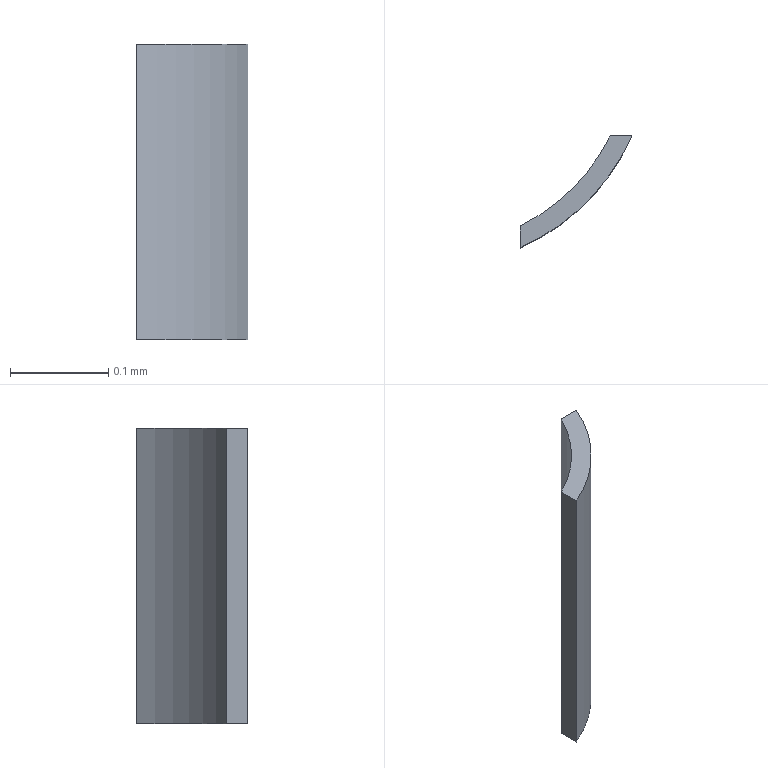Part | STEP file | RJ-USIO-V1_2-220411_172 | 1 solid | 6 faces | box 0.1135 x 0.1135 x 0.3 mm | volume 0.0008879 mm3 | plane 4 | cylinder 2 | commonest cylinder face diameters 0.4 x1 0.44 x1
STEP:
#1=CARTESIAN_POINT('',(0.,0.,0.));
#2=DIRECTION('',(0.,0.,1.));
#3=DIRECTION('',(1.,0.,0.));
#4=AXIS2_PLACEMENT_3D('',#1,#2,#3);
#5=CARTESIAN_POINT('',(38.2,55.808,0.02));
#6=VERTEX_POINT('',#5);
#7=CARTESIAN_POINT('',(38.291,55.9,0.02));
#8=VERTEX_POINT('',#7);
#9=CARTESIAN_POINT('',(38.112,55.988,0.02));
#10=DIRECTION('',(0.,-0.000000044,1.));
#11=DIRECTION('',(0.4406,-0.8977,-0.000000039));
#12=AXIS2_PLACEMENT_3D('',#9,#10,#11);
#13=CIRCLE('',#12,0.2);
#14=CARTESIAN_POINT('',(38.112,55.988,0.02));
#15=DIRECTION('',(0.,-0.000000044,1.));
#16=DIRECTION('',(-0.000000175,1.,0.000000044));
#17=AXIS2_PLACEMENT_3D('',#14,#15,#16);
#18=PLANE('',#17);
#19=CARTESIAN_POINT('',(0.,0.));
#20=DIRECTION('',(-0.8977,-0.4406));
#21=AXIS2_PLACEMENT_2D('',#19,#20);
#22=CIRCLE('',#21,0.2);
#23=(GEOMETRIC_REPRESENTATION_CONTEXT(2)PARAMETRIC_REPRESENTATION_CONTEXT()REPRESENTATION_CONTEXT('',''));
#24=DEFINITIONAL_REPRESENTATION('',(#22),#23);
#25=PCURVE('',#18,#24);
#26=CARTESIAN_POINT('',(38.112,55.988,0.32));
#27=DIRECTION('',(0.,0.000000044,-1.));
#28=DIRECTION('',(0.000000175,-1.,-0.000000044));
#29=AXIS2_PLACEMENT_3D('',#26,#27,#28);
#30=CYLINDRICAL_SURFACE('',#29,0.2);
#31=CARTESIAN_POINT('',(5.827,0.3));
#32=DIRECTION('',(-1.,0.));
#33=VECTOR('',#32,1.);
#34=LINE('',#31,#33);
#35=(GEOMETRIC_REPRESENTATION_CONTEXT(2)PARAMETRIC_REPRESENTATION_CONTEXT()REPRESENTATION_CONTEXT('',''));
#36=DEFINITIONAL_REPRESENTATION('',(#34),#35);
#37=PCURVE('',#30,#36);
#38=SURFACE_CURVE('',#13,(#25,#37),.PCURVE_S1.);
#39=EDGE_CURVE('',#6,#8,#38,.T.);
#40=ORIENTED_EDGE('',*,*,#39,.F.);
#41=CARTESIAN_POINT('',(38.2,55.786,0.02));
#42=VERTEX_POINT('',#41);
#43=CARTESIAN_POINT('',(38.2,55.786,0.02));
#44=DIRECTION('',(-0.000000175,1.,0.000000044));
#45=VECTOR('',#44,1.);
#46=LINE('',#43,#45);
#47=CARTESIAN_POINT('',(-0.2016,-0.08812));
#48=DIRECTION('',(1.,0.));
#49=VECTOR('',#48,1.);
#50=LINE('',#47,#49);
#51=(GEOMETRIC_REPRESENTATION_CONTEXT(2)PARAMETRIC_REPRESENTATION_CONTEXT()REPRESENTATION_CONTEXT('',''));
#52=DEFINITIONAL_REPRESENTATION('',(#50),#51);
#53=PCURVE('',#18,#52);
#54=CARTESIAN_POINT('',(38.2,55.808,0.32));
#55=DIRECTION('',(1.,0.000000175,0.));
#56=DIRECTION('',(0.000000175,-1.,-0.000000044));
#57=AXIS2_PLACEMENT_3D('',#54,#55,#56);
#58=PLANE('',#57);
#59=CARTESIAN_POINT('',(0.02204,0.3));
#60=DIRECTION('',(-1.,0.));
#61=VECTOR('',#60,1.);
#62=LINE('',#59,#61);
#63=(GEOMETRIC_REPRESENTATION_CONTEXT(2)PARAMETRIC_REPRESENTATION_CONTEXT()REPRESENTATION_CONTEXT('',''));
#64=DEFINITIONAL_REPRESENTATION('',(#62),#63);
#65=PCURVE('',#58,#64);
#66=SURFACE_CURVE('',#46,(#53,#65),.PCURVE_S1.);
#67=EDGE_CURVE('',#42,#6,#66,.T.);
#68=ORIENTED_EDGE('',*,*,#67,.F.);
#69=CARTESIAN_POINT('',(38.313,55.9,0.02));
#70=VERTEX_POINT('',#69);
#71=CARTESIAN_POINT('',(38.112,55.988,0.02));
#72=DIRECTION('',(0.,0.000000044,-1.));
#73=DIRECTION('',(0.9163,-0.4005,-0.000000018));
#74=AXIS2_PLACEMENT_3D('',#71,#72,#73);
#75=CIRCLE('',#74,0.22);
#76=CARTESIAN_POINT('',(-0.08812,-0.2016));
#77=CARTESIAN_POINT('',(-0.4373,-0.04895));
#78=CARTESIAN_POINT('',(-0.1305,0.1771));
#79=CARTESIAN_POINT('',(0.1762,0.4032));
#80=CARTESIAN_POINT('',(0.2186,0.02448));
#81=CARTESIAN_POINT('',(0.261,-0.3542));
#82=CARTESIAN_POINT('',(-0.08812,-0.2016));
#83=(BOUNDED_CURVE()B_SPLINE_CURVE(2,(#76,#77,#78,#79,#80,#81,#82),.UNSPECIFIED.,.T.,.F.)B_SPLINE_CURVE_WITH_KNOTS((1,2,2,2,2,1),(-2.094,0.,2.094,4.189,6.283,8.378),.UNSPECIFIED.)CURVE()GEOMETRIC_REPRESENTATION_ITEM()RATIONAL_B_SPLINE_CURVE((1.,0.5,1.,0.5,1.,0.5,1.))REPRESENTATION_ITEM(''));
#84=(GEOMETRIC_REPRESENTATION_CONTEXT(2)PARAMETRIC_REPRESENTATION_CONTEXT()REPRESENTATION_CONTEXT('',''));
#85=DEFINITIONAL_REPRESENTATION('',(#83),#84);
#86=PCURVE('',#18,#85);
#87=CARTESIAN_POINT('',(38.112,55.988,0.32));
#88=DIRECTION('',(0.,0.000000044,-1.));
#89=DIRECTION('',(0.000000175,-1.,-0.000000044));
#90=AXIS2_PLACEMENT_3D('',#87,#88,#89);
#91=CYLINDRICAL_SURFACE('',#90,0.22);
#92=CARTESIAN_POINT('',(5.124,0.3));
#93=DIRECTION('',(1.,0.));
#94=VECTOR('',#93,1.);
#95=LINE('',#92,#94);
#96=(GEOMETRIC_REPRESENTATION_CONTEXT(2)PARAMETRIC_REPRESENTATION_CONTEXT()REPRESENTATION_CONTEXT('',''));
#97=DEFINITIONAL_REPRESENTATION('',(#95),#96);
#98=PCURVE('',#91,#97);
#99=SURFACE_CURVE('',#75,(#86,#98),.PCURVE_S1.);
#100=EDGE_CURVE('',#70,#42,#99,.T.);
#101=ORIENTED_EDGE('',*,*,#100,.F.);
#102=CARTESIAN_POINT('',(38.291,55.9,0.02));
#103=DIRECTION('',(1.,0.000000175,0.));
#104=VECTOR('',#103,1.);
#105=LINE('',#102,#104);
#106=CARTESIAN_POINT('',(-0.08812,-0.1795));
#107=DIRECTION('',(0.,-1.));
#108=VECTOR('',#107,1.);
#109=LINE('',#106,#108);
#110=(GEOMETRIC_REPRESENTATION_CONTEXT(2)PARAMETRIC_REPRESENTATION_CONTEXT()REPRESENTATION_CONTEXT('',''));
#111=DEFINITIONAL_REPRESENTATION('',(#109),#110);
#112=PCURVE('',#18,#111);
#113=CARTESIAN_POINT('',(38.291,55.9,0.32));
#114=DIRECTION('',(0.000000175,-1.,-0.000000044));
#115=DIRECTION('',(-1.,-0.000000175,0.));
#116=AXIS2_PLACEMENT_3D('',#113,#114,#115);
#117=PLANE('',#116);
#118=CARTESIAN_POINT('',(0.,0.3));
#119=DIRECTION('',(-1.,0.));
#120=VECTOR('',#119,1.);
#121=LINE('',#118,#120);
#122=(GEOMETRIC_REPRESENTATION_CONTEXT(2)PARAMETRIC_REPRESENTATION_CONTEXT()REPRESENTATION_CONTEXT('',''));
#123=DEFINITIONAL_REPRESENTATION('',(#121),#122);
#124=PCURVE('',#117,#123);
#125=SURFACE_CURVE('',#105,(#112,#124),.PCURVE_S1.);
#126=EDGE_CURVE('',#8,#70,#125,.T.);
#127=ORIENTED_EDGE('',*,*,#126,.F.);
#128=EDGE_LOOP('',(#40,#68,#101,#127));
#129=FACE_BOUND('',#128,.F.);
#130=ADVANCED_FACE('',(#129),#18,.F.);
#131=ORIENTED_EDGE('',*,*,#39,.T.);
#132=CARTESIAN_POINT('',(38.291,55.9,0.32));
#133=VERTEX_POINT('',#132);
#134=CARTESIAN_POINT('',(38.291,55.9,0.32));
#135=DIRECTION('',(0.,0.000000044,-1.));
#136=VECTOR('',#135,1.);
#137=LINE('',#134,#136);
#138=CARTESIAN_POINT('',(5.169,0.));
#139=DIRECTION('',(0.,1.));
#140=VECTOR('',#139,1.);
#141=LINE('',#138,#140);
#142=(GEOMETRIC_REPRESENTATION_CONTEXT(2)PARAMETRIC_REPRESENTATION_CONTEXT()REPRESENTATION_CONTEXT('',''));
#143=DEFINITIONAL_REPRESENTATION('',(#141),#142);
#144=PCURVE('',#30,#143);
#145=CARTESIAN_POINT('',(0.,0.));
#146=DIRECTION('',(0.,1.));
#147=VECTOR('',#146,1.);
#148=LINE('',#145,#147);
#149=(GEOMETRIC_REPRESENTATION_CONTEXT(2)PARAMETRIC_REPRESENTATION_CONTEXT()REPRESENTATION_CONTEXT('',''));
#150=DEFINITIONAL_REPRESENTATION('',(#148),#149);
#151=PCURVE('',#117,#150);
#152=SURFACE_CURVE('',#137,(#144,#151),.PCURVE_S1.);
#153=EDGE_CURVE('',#133,#8,#152,.T.);
#154=ORIENTED_EDGE('',*,*,#153,.F.);
#155=CARTESIAN_POINT('',(38.2,55.808,0.32));
#156=VERTEX_POINT('',#155);
#157=CARTESIAN_POINT('',(38.112,55.988,0.32));
#158=DIRECTION('',(0.,0.000000044,-1.));
#159=DIRECTION('',(0.8977,-0.4406,-0.000000019));
#160=AXIS2_PLACEMENT_3D('',#157,#158,#159);
#161=CIRCLE('',#160,0.2);
#162=CARTESIAN_POINT('',(5.169,0.));
#163=DIRECTION('',(1.,0.));
#164=VECTOR('',#163,1.);
#165=LINE('',#162,#164);
#166=(GEOMETRIC_REPRESENTATION_CONTEXT(2)PARAMETRIC_REPRESENTATION_CONTEXT()REPRESENTATION_CONTEXT('',''));
#167=DEFINITIONAL_REPRESENTATION('',(#165),#166);
#168=PCURVE('',#30,#167);
#169=CARTESIAN_POINT('',(38.112,55.988,0.32));
#170=DIRECTION('',(0.,-0.000000044,1.));
#171=DIRECTION('',(-0.000000175,1.,0.000000044));
#172=AXIS2_PLACEMENT_3D('',#169,#170,#171);
#173=PLANE('',#172);
#174=CARTESIAN_POINT('',(-0.08812,-0.1795));
#175=CARTESIAN_POINT('',(-0.3991,-0.02691));
#176=CARTESIAN_POINT('',(-0.1114,0.1661));
#177=CARTESIAN_POINT('',(0.1762,0.3591));
#178=CARTESIAN_POINT('',(0.1995,0.01346));
#179=CARTESIAN_POINT('',(0.2229,-0.3322));
#180=CARTESIAN_POINT('',(-0.08812,-0.1795));
#181=(BOUNDED_CURVE()B_SPLINE_CURVE(2,(#174,#175,#176,#177,#178,#179,#180),.UNSPECIFIED.,.T.,.F.)B_SPLINE_CURVE_WITH_KNOTS((1,2,2,2,2,1),(-2.094,0.,2.094,4.189,6.283,8.378),.UNSPECIFIED.)CURVE()GEOMETRIC_REPRESENTATION_ITEM()RATIONAL_B_SPLINE_CURVE((1.,0.5,1.,0.5,1.,0.5,1.))REPRESENTATION_ITEM(''));
#182=(GEOMETRIC_REPRESENTATION_CONTEXT(2)PARAMETRIC_REPRESENTATION_CONTEXT()REPRESENTATION_CONTEXT('',''));
#183=DEFINITIONAL_REPRESENTATION('',(#181),#182);
#184=PCURVE('',#173,#183);
#185=SURFACE_CURVE('',#161,(#168,#184),.PCURVE_S1.);
#186=EDGE_CURVE('',#133,#156,#185,.T.);
#187=ORIENTED_EDGE('',*,*,#186,.T.);
#188=CARTESIAN_POINT('',(38.2,55.808,0.02));
#189=DIRECTION('',(0.,-0.000000044,1.));
#190=VECTOR('',#189,1.);
#191=LINE('',#188,#190);
#192=CARTESIAN_POINT('',(5.827,0.3));
#193=DIRECTION('',(0.,-1.));
#194=VECTOR('',#193,1.);
#195=LINE('',#192,#194);
#196=(GEOMETRIC_REPRESENTATION_CONTEXT(2)PARAMETRIC_REPRESENTATION_CONTEXT()REPRESENTATION_CONTEXT('',''));
#197=DEFINITIONAL_REPRESENTATION('',(#195),#196);
#198=PCURVE('',#30,#197);
#199=CARTESIAN_POINT('',(0.,0.3));
#200=DIRECTION('',(0.,-1.));
#201=VECTOR('',#200,1.);
#202=LINE('',#199,#201);
#203=(GEOMETRIC_REPRESENTATION_CONTEXT(2)PARAMETRIC_REPRESENTATION_CONTEXT()REPRESENTATION_CONTEXT('',''));
#204=DEFINITIONAL_REPRESENTATION('',(#202),#203);
#205=PCURVE('',#58,#204);
#206=SURFACE_CURVE('',#191,(#198,#205),.PCURVE_S1.);
#207=EDGE_CURVE('',#6,#156,#206,.T.);
#208=ORIENTED_EDGE('',*,*,#207,.F.);
#209=EDGE_LOOP('',(#131,#154,#187,#208));
#210=FACE_BOUND('',#209,.F.);
#211=ADVANCED_FACE('',(#210),#30,.F.);
#212=ORIENTED_EDGE('',*,*,#126,.T.);
#213=CARTESIAN_POINT('',(38.313,55.9,0.32));
#214=VERTEX_POINT('',#213);
#215=CARTESIAN_POINT('',(38.313,55.9,0.02));
#216=DIRECTION('',(0.,-0.000000044,1.));
#217=VECTOR('',#216,1.);
#218=LINE('',#215,#217);
#219=CARTESIAN_POINT('',(-0.02204,0.3));
#220=DIRECTION('',(0.,-1.));
#221=VECTOR('',#220,1.);
#222=LINE('',#219,#221);
#223=(GEOMETRIC_REPRESENTATION_CONTEXT(2)PARAMETRIC_REPRESENTATION_CONTEXT()REPRESENTATION_CONTEXT('',''));
#224=DEFINITIONAL_REPRESENTATION('',(#222),#223);
#225=PCURVE('',#117,#224);
#226=CARTESIAN_POINT('',(5.124,0.3));
#227=DIRECTION('',(0.,-1.));
#228=VECTOR('',#227,1.);
#229=LINE('',#226,#228);
#230=(GEOMETRIC_REPRESENTATION_CONTEXT(2)PARAMETRIC_REPRESENTATION_CONTEXT()REPRESENTATION_CONTEXT('',''));
#231=DEFINITIONAL_REPRESENTATION('',(#229),#230);
#232=PCURVE('',#91,#231);
#233=SURFACE_CURVE('',#218,(#225,#232),.PCURVE_S1.);
#234=EDGE_CURVE('',#70,#214,#233,.T.);
#235=ORIENTED_EDGE('',*,*,#234,.T.);
#236=CARTESIAN_POINT('',(38.291,55.9,0.32));
#237=DIRECTION('',(1.,0.000000175,0.));
#238=VECTOR('',#237,1.);
#239=LINE('',#236,#238);
#240=CARTESIAN_POINT('',(0.,0.));
#241=DIRECTION('',(-1.,0.));
#242=VECTOR('',#241,1.);
#243=LINE('',#240,#242);
#244=(GEOMETRIC_REPRESENTATION_CONTEXT(2)PARAMETRIC_REPRESENTATION_CONTEXT()REPRESENTATION_CONTEXT('',''));
#245=DEFINITIONAL_REPRESENTATION('',(#243),#244);
#246=PCURVE('',#117,#245);
#247=CARTESIAN_POINT('',(-0.08812,-0.1795));
#248=DIRECTION('',(0.,-1.));
#249=VECTOR('',#248,1.);
#250=LINE('',#247,#249);
#251=(GEOMETRIC_REPRESENTATION_CONTEXT(2)PARAMETRIC_REPRESENTATION_CONTEXT()REPRESENTATION_CONTEXT('',''));
#252=DEFINITIONAL_REPRESENTATION('',(#250),#251);
#253=PCURVE('',#173,#252);
#254=SURFACE_CURVE('',#239,(#246,#253),.PCURVE_S1.);
#255=EDGE_CURVE('',#133,#214,#254,.T.);
#256=ORIENTED_EDGE('',*,*,#255,.F.);
#257=ORIENTED_EDGE('',*,*,#153,.T.);
#258=EDGE_LOOP('',(#212,#235,#256,#257));
#259=FACE_BOUND('',#258,.F.);
#260=ADVANCED_FACE('',(#259),#117,.F.);
#261=ORIENTED_EDGE('',*,*,#234,.T.);
#262=CARTESIAN_POINT('',(38.2,55.786,0.32));
#263=VERTEX_POINT('',#262);
#264=CARTESIAN_POINT('',(38.112,55.988,0.32));
#265=DIRECTION('',(0.,-0.000000044,1.));
#266=DIRECTION('',(0.4005,-0.9163,-0.00000004));
#267=AXIS2_PLACEMENT_3D('',#264,#265,#266);
#268=CIRCLE('',#267,0.22);
#269=CARTESIAN_POINT('',(5.871,0.));
#270=DIRECTION('',(-1.,0.));
#271=VECTOR('',#270,1.);
#272=LINE('',#269,#271);
#273=(GEOMETRIC_REPRESENTATION_CONTEXT(2)PARAMETRIC_REPRESENTATION_CONTEXT()REPRESENTATION_CONTEXT('',''));
#274=DEFINITIONAL_REPRESENTATION('',(#272),#273);
#275=PCURVE('',#91,#274);
#276=CARTESIAN_POINT('',(0.,0.));
#277=DIRECTION('',(-0.9163,-0.4005));
#278=AXIS2_PLACEMENT_2D('',#276,#277);
#279=CIRCLE('',#278,0.22);
#280=(GEOMETRIC_REPRESENTATION_CONTEXT(2)PARAMETRIC_REPRESENTATION_CONTEXT()REPRESENTATION_CONTEXT('',''));
#281=DEFINITIONAL_REPRESENTATION('',(#279),#280);
#282=PCURVE('',#173,#281);
#283=SURFACE_CURVE('',#268,(#275,#282),.PCURVE_S1.);
#284=EDGE_CURVE('',#263,#214,#283,.T.);
#285=ORIENTED_EDGE('',*,*,#284,.F.);
#286=CARTESIAN_POINT('',(38.2,55.786,0.32));
#287=DIRECTION('',(0.,0.000000044,-1.));
#288=VECTOR('',#287,1.);
#289=LINE('',#286,#288);
#290=CARTESIAN_POINT('',(5.871,0.));
#291=DIRECTION('',(0.,1.));
#292=VECTOR('',#291,1.);
#293=LINE('',#290,#292);
#294=(GEOMETRIC_REPRESENTATION_CONTEXT(2)PARAMETRIC_REPRESENTATION_CONTEXT()REPRESENTATION_CONTEXT('',''));
#295=DEFINITIONAL_REPRESENTATION('',(#293),#294);
#296=PCURVE('',#91,#295);
#297=CARTESIAN_POINT('',(0.02204,0.));
#298=DIRECTION('',(0.,1.));
#299=VECTOR('',#298,1.);
#300=LINE('',#297,#299);
#301=(GEOMETRIC_REPRESENTATION_CONTEXT(2)PARAMETRIC_REPRESENTATION_CONTEXT()REPRESENTATION_CONTEXT('',''));
#302=DEFINITIONAL_REPRESENTATION('',(#300),#301);
#303=PCURVE('',#58,#302);
#304=SURFACE_CURVE('',#289,(#296,#303),.PCURVE_S1.);
#305=EDGE_CURVE('',#263,#42,#304,.T.);
#306=ORIENTED_EDGE('',*,*,#305,.T.);
#307=ORIENTED_EDGE('',*,*,#100,.F.);
#308=EDGE_LOOP('',(#261,#285,#306,#307));
#309=FACE_BOUND('',#308,.T.);
#310=ADVANCED_FACE('',(#309),#91,.T.);
#311=ORIENTED_EDGE('',*,*,#67,.T.);
#312=ORIENTED_EDGE('',*,*,#207,.T.);
#313=CARTESIAN_POINT('',(38.2,55.786,0.32));
#314=DIRECTION('',(-0.000000175,1.,0.000000044));
#315=VECTOR('',#314,1.);
#316=LINE('',#313,#315);
#317=CARTESIAN_POINT('',(0.02204,0.));
#318=DIRECTION('',(-1.,0.));
#319=VECTOR('',#318,1.);
#320=LINE('',#317,#319);
#321=(GEOMETRIC_REPRESENTATION_CONTEXT(2)PARAMETRIC_REPRESENTATION_CONTEXT()REPRESENTATION_CONTEXT('',''));
#322=DEFINITIONAL_REPRESENTATION('',(#320),#321);
#323=PCURVE('',#58,#322);
#324=CARTESIAN_POINT('',(-0.2016,-0.08812));
#325=DIRECTION('',(1.,0.));
#326=VECTOR('',#325,1.);
#327=LINE('',#324,#326);
#328=(GEOMETRIC_REPRESENTATION_CONTEXT(2)PARAMETRIC_REPRESENTATION_CONTEXT()REPRESENTATION_CONTEXT('',''));
#329=DEFINITIONAL_REPRESENTATION('',(#327),#328);
#330=PCURVE('',#173,#329);
#331=SURFACE_CURVE('',#316,(#323,#330),.PCURVE_S1.);
#332=EDGE_CURVE('',#263,#156,#331,.T.);
#333=ORIENTED_EDGE('',*,*,#332,.F.);
#334=ORIENTED_EDGE('',*,*,#305,.T.);
#335=EDGE_LOOP('',(#311,#312,#333,#334));
#336=FACE_BOUND('',#335,.F.);
#337=ADVANCED_FACE('',(#336),#58,.F.);
#338=ORIENTED_EDGE('',*,*,#186,.F.);
#339=ORIENTED_EDGE('',*,*,#255,.T.);
#340=ORIENTED_EDGE('',*,*,#284,.F.);
#341=ORIENTED_EDGE('',*,*,#332,.T.);
#342=EDGE_LOOP('',(#338,#339,#340,#341));
#343=FACE_BOUND('',#342,.F.);
#344=ADVANCED_FACE('',(#343),#173,.T.);
#345=CLOSED_SHELL('',(#130,#211,#260,#310,#337,#344));
#346=MANIFOLD_SOLID_BREP('',#345);
#347=(LENGTH_UNIT()NAMED_UNIT(*)SI_UNIT(.MILLI.,.METRE.));
#348=UNCERTAINTY_MEASURE_WITH_UNIT(LENGTH_MEASURE(0.0000001),#347,'','');
#349=(NAMED_UNIT(*)PLANE_ANGLE_UNIT()SI_UNIT($,.RADIAN.));
#350=(NAMED_UNIT(*)SI_UNIT($,.STERADIAN.)SOLID_ANGLE_UNIT());
#351=(GEOMETRIC_REPRESENTATION_CONTEXT(3)GLOBAL_UNCERTAINTY_ASSIGNED_CONTEXT((#348))GLOBAL_UNIT_ASSIGNED_CONTEXT((#347,#349,#350))REPRESENTATION_CONTEXT('',''));
#352=ADVANCED_BREP_SHAPE_REPRESENTATION('',(#4,#346),#351);